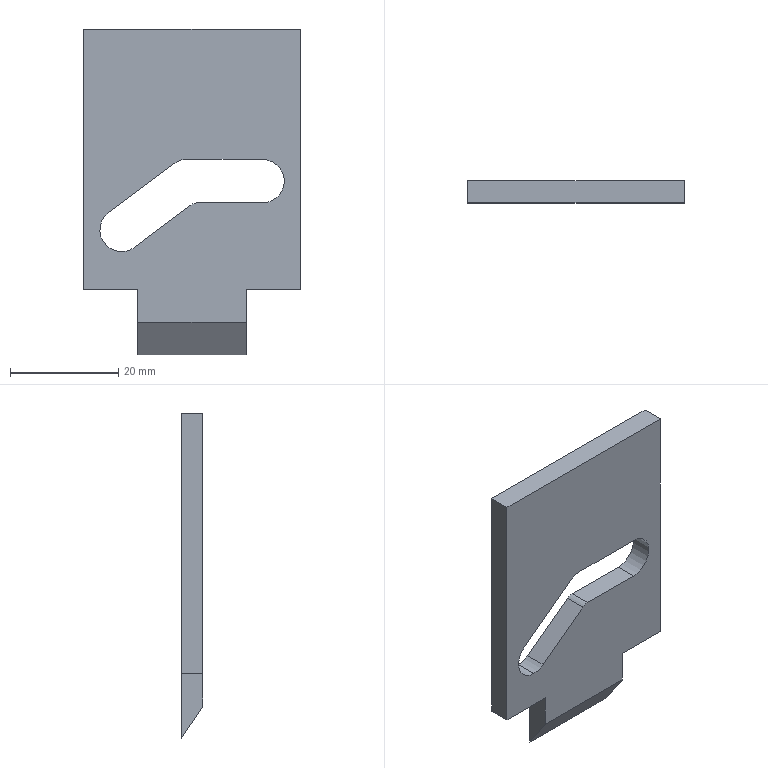Part | SolidWorks | features BaseBody 1 | 1 solid | 19 faces | box 40 x 4 x 60 mm | volume 7271 mm3 | plane 14 | cylinder 5 | commonest cylinder face diameters 8 x4 4 x1
STEP:
#1=CARTESIAN_POINT('',(-13.,4.,-17.));
#2=VERTEX_POINT('',#1);
#3=CARTESIAN_POINT('',(-10.6,4.,-16.2));
#4=VERTEX_POINT('',#3);
#5=CARTESIAN_POINT('',(-13.,4.,-13.));
#6=DIRECTION('',(0.,-1.,0.));
#7=DIRECTION('',(0.,0.,-1.));
#8=AXIS2_PLACEMENT_3D('',#5,#6,#7);
#9=CIRCLE('',#8,4.);
#10=EDGE_CURVE('',#2,#4,#9,.T.);
#11=ORIENTED_EDGE('',*,*,#10,.F.);
#12=CARTESIAN_POINT('',(-13.,0.,-17.));
#13=VERTEX_POINT('',#12);
#14=CARTESIAN_POINT('',(-13.,4.,-17.));
#15=DIRECTION('',(0.,-1.,0.));
#16=VECTOR('',#15,1000.);
#17=LINE('',#14,#16);
#18=EDGE_CURVE('',#2,#13,#17,.T.);
#19=ORIENTED_EDGE('',*,*,#18,.T.);
#20=CARTESIAN_POINT('',(-10.6,0.,-16.2));
#21=VERTEX_POINT('',#20);
#22=CARTESIAN_POINT('',(-13.,0.,-13.));
#23=DIRECTION('',(0.,1.,0.));
#24=DIRECTION('',(0.,0.,-1.));
#25=AXIS2_PLACEMENT_3D('',#22,#23,#24);
#26=CIRCLE('',#25,4.);
#27=EDGE_CURVE('',#21,#13,#26,.T.);
#28=ORIENTED_EDGE('',*,*,#27,.F.);
#29=CARTESIAN_POINT('',(-10.6,4.,-16.2));
#30=DIRECTION('',(0.,-1.,0.));
#31=VECTOR('',#30,1000.);
#32=LINE('',#29,#31);
#33=EDGE_CURVE('',#4,#21,#32,.T.);
#34=ORIENTED_EDGE('',*,*,#33,.F.);
#35=EDGE_LOOP('',(#11,#19,#28,#34));
#36=FACE_OUTER_BOUND('',#35,.T.);
#37=CARTESIAN_POINT('',(-13.,4.,-13.));
#38=DIRECTION('',(0.,-1.,0.));
#39=DIRECTION('',(0.,0.,-1.));
#40=AXIS2_PLACEMENT_3D('',#37,#38,#39);
#41=CYLINDRICAL_SURFACE('',#40,4.);
#42=ADVANCED_FACE('',(#36),#41,.F.);
#43=CARTESIAN_POINT('',(-15.4,4.,-9.8));
#44=VERTEX_POINT('',#43);
#45=CARTESIAN_POINT('',(-13.,4.,-13.));
#46=DIRECTION('',(0.,-1.,0.));
#47=DIRECTION('',(0.,0.,-1.));
#48=AXIS2_PLACEMENT_3D('',#45,#46,#47);
#49=CIRCLE('',#48,4.);
#50=EDGE_CURVE('',#44,#2,#49,.T.);
#51=ORIENTED_EDGE('',*,*,#50,.T.);
#52=ORIENTED_EDGE('',*,*,#10,.T.);
#53=CARTESIAN_POINT('',(-0.2,4.,-8.4));
#54=VERTEX_POINT('',#53);
#55=CARTESIAN_POINT('',(-10.6,4.,-16.2));
#56=DIRECTION('',(0.8,0.,0.6));
#57=VECTOR('',#56,1000.);
#58=LINE('',#55,#57);
#59=EDGE_CURVE('',#4,#54,#58,.T.);
#60=ORIENTED_EDGE('',*,*,#59,.T.);
#61=CARTESIAN_POINT('',(1.,4.,-8.));
#62=VERTEX_POINT('',#61);
#63=CARTESIAN_POINT('',(1.,4.,-10.));
#64=DIRECTION('',(0.,-1.,0.));
#65=DIRECTION('',(0.,0.,-1.));
#66=AXIS2_PLACEMENT_3D('',#63,#64,#65);
#67=CIRCLE('',#66,2.);
#68=EDGE_CURVE('',#62,#54,#67,.T.);
#69=ORIENTED_EDGE('',*,*,#68,.F.);
#70=CARTESIAN_POINT('',(13.,4.,-8.));
#71=VERTEX_POINT('',#70);
#72=CARTESIAN_POINT('',(0.,4.,-8.));
#73=DIRECTION('',(1.,0.,0.));
#74=VECTOR('',#73,1000.);
#75=LINE('',#72,#74);
#76=EDGE_CURVE('',#62,#71,#75,.T.);
#77=ORIENTED_EDGE('',*,*,#76,.T.);
#78=CARTESIAN_POINT('',(13.,4.,0.));
#79=VERTEX_POINT('',#78);
#80=CARTESIAN_POINT('',(13.,4.,-4.));
#81=DIRECTION('',(0.,-1.,0.));
#82=DIRECTION('',(0.,0.,-1.));
#83=AXIS2_PLACEMENT_3D('',#80,#81,#82);
#84=CIRCLE('',#83,4.);
#85=EDGE_CURVE('',#71,#79,#84,.T.);
#86=ORIENTED_EDGE('',*,*,#85,.T.);
#87=CARTESIAN_POINT('',(-1.,4.,0.));
#88=VERTEX_POINT('',#87);
#89=CARTESIAN_POINT('',(0.,4.,0.));
#90=DIRECTION('',(-1.,0.,0.));
#91=VECTOR('',#90,1000.);
#92=LINE('',#89,#91);
#93=EDGE_CURVE('',#79,#88,#92,.T.);
#94=ORIENTED_EDGE('',*,*,#93,.T.);
#95=CARTESIAN_POINT('',(-3.4,4.,-0.8));
#96=VERTEX_POINT('',#95);
#97=CARTESIAN_POINT('',(-1.,4.,-4.));
#98=DIRECTION('',(0.,-1.,0.));
#99=DIRECTION('',(0.,0.,-1.));
#100=AXIS2_PLACEMENT_3D('',#97,#98,#99);
#101=CIRCLE('',#100,4.);
#102=EDGE_CURVE('',#88,#96,#101,.T.);
#103=ORIENTED_EDGE('',*,*,#102,.T.);
#104=CARTESIAN_POINT('',(-3.4,4.,-0.8));
#105=DIRECTION('',(-0.8,0.,-0.6));
#106=VECTOR('',#105,1000.);
#107=LINE('',#104,#106);
#108=EDGE_CURVE('',#96,#44,#107,.T.);
#109=ORIENTED_EDGE('',*,*,#108,.T.);
#110=EDGE_LOOP('',(#51,#52,#60,#69,#77,#86,#94,#103,#109));
#111=FACE_BOUND('',#110,.T.);
#112=CARTESIAN_POINT('',(20.,4.,24.));
#113=VERTEX_POINT('',#112);
#114=CARTESIAN_POINT('',(20.,4.,-24.));
#115=VERTEX_POINT('',#114);
#116=CARTESIAN_POINT('',(20.,4.,0.));
#117=DIRECTION('',(0.,0.,-1.));
#118=VECTOR('',#117,1000.);
#119=LINE('',#116,#118);
#120=EDGE_CURVE('',#113,#115,#119,.T.);
#121=ORIENTED_EDGE('',*,*,#120,.T.);
#122=CARTESIAN_POINT('',(10.,4.,-24.));
#123=VERTEX_POINT('',#122);
#124=CARTESIAN_POINT('',(0.,4.,-24.));
#125=DIRECTION('',(-1.,0.,0.));
#126=VECTOR('',#125,1000.);
#127=LINE('',#124,#126);
#128=EDGE_CURVE('',#115,#123,#127,.T.);
#129=ORIENTED_EDGE('',*,*,#128,.T.);
#130=CARTESIAN_POINT('',(10.,4.,-36.));
#131=VERTEX_POINT('',#130);
#132=CARTESIAN_POINT('',(10.,4.,0.));
#133=DIRECTION('',(0.,0.,-1.));
#134=VECTOR('',#133,1000.);
#135=LINE('',#132,#134);
#136=EDGE_CURVE('',#123,#131,#135,.T.);
#137=ORIENTED_EDGE('',*,*,#136,.T.);
#138=CARTESIAN_POINT('',(-10.,4.,-36.));
#139=VERTEX_POINT('',#138);
#140=CARTESIAN_POINT('',(0.,4.,-36.));
#141=DIRECTION('',(-1.,0.,0.));
#142=VECTOR('',#141,1000.);
#143=LINE('',#140,#142);
#144=EDGE_CURVE('',#131,#139,#143,.T.);
#145=ORIENTED_EDGE('',*,*,#144,.T.);
#146=CARTESIAN_POINT('',(-10.,4.,-24.));
#147=VERTEX_POINT('',#146);
#148=CARTESIAN_POINT('',(-10.,4.,0.));
#149=DIRECTION('',(0.,0.,1.));
#150=VECTOR('',#149,1000.);
#151=LINE('',#148,#150);
#152=EDGE_CURVE('',#139,#147,#151,.T.);
#153=ORIENTED_EDGE('',*,*,#152,.T.);
#154=CARTESIAN_POINT('',(-20.,4.,-24.));
#155=VERTEX_POINT('',#154);
#156=CARTESIAN_POINT('',(0.,4.,-24.));
#157=DIRECTION('',(-1.,0.,0.));
#158=VECTOR('',#157,1000.);
#159=LINE('',#156,#158);
#160=EDGE_CURVE('',#147,#155,#159,.T.);
#161=ORIENTED_EDGE('',*,*,#160,.T.);
#162=CARTESIAN_POINT('',(-20.,4.,24.));
#163=VERTEX_POINT('',#162);
#164=CARTESIAN_POINT('',(-20.,4.,0.));
#165=DIRECTION('',(0.,0.,1.));
#166=VECTOR('',#165,1000.);
#167=LINE('',#164,#166);
#168=EDGE_CURVE('',#155,#163,#167,.T.);
#169=ORIENTED_EDGE('',*,*,#168,.T.);
#170=CARTESIAN_POINT('',(0.,4.,24.));
#171=DIRECTION('',(1.,0.,0.));
#172=VECTOR('',#171,1000.);
#173=LINE('',#170,#172);
#174=EDGE_CURVE('',#163,#113,#173,.T.);
#175=ORIENTED_EDGE('',*,*,#174,.T.);
#176=EDGE_LOOP('',(#121,#129,#137,#145,#153,#161,#169,#175));
#177=FACE_OUTER_BOUND('',#176,.T.);
#178=CARTESIAN_POINT('',(0.,4.,0.));
#179=DIRECTION('',(0.,1.,0.));
#180=DIRECTION('',(0.,0.,1.));
#181=AXIS2_PLACEMENT_3D('',#178,#179,#180);
#182=PLANE('',#181);
#183=ADVANCED_FACE('',(#111,#177),#182,.T.);
#184=ORIENTED_EDGE('',*,*,#18,.F.);
#185=ORIENTED_EDGE('',*,*,#50,.F.);
#186=CARTESIAN_POINT('',(-15.4,0.,-9.8));
#187=VERTEX_POINT('',#186);
#188=CARTESIAN_POINT('',(-15.4,4.,-9.8));
#189=DIRECTION('',(0.,1.,0.));
#190=VECTOR('',#189,1000.);
#191=LINE('',#188,#190);
#192=EDGE_CURVE('',#187,#44,#191,.T.);
#193=ORIENTED_EDGE('',*,*,#192,.F.);
#194=CARTESIAN_POINT('',(-13.,0.,-13.));
#195=DIRECTION('',(0.,1.,0.));
#196=DIRECTION('',(0.,0.,-1.));
#197=AXIS2_PLACEMENT_3D('',#194,#195,#196);
#198=CIRCLE('',#197,4.);
#199=EDGE_CURVE('',#13,#187,#198,.T.);
#200=ORIENTED_EDGE('',*,*,#199,.F.);
#201=EDGE_LOOP('',(#184,#185,#193,#200));
#202=FACE_OUTER_BOUND('',#201,.T.);
#203=CARTESIAN_POINT('',(-13.,4.,-13.));
#204=DIRECTION('',(0.,-1.,0.));
#205=DIRECTION('',(0.,0.,-1.));
#206=AXIS2_PLACEMENT_3D('',#203,#204,#205);
#207=CYLINDRICAL_SURFACE('',#206,4.);
#208=ADVANCED_FACE('',(#202),#207,.F.);
#209=ORIENTED_EDGE('',*,*,#192,.T.);
#210=ORIENTED_EDGE('',*,*,#108,.F.);
#211=CARTESIAN_POINT('',(-3.4,0.,-0.8));
#212=VERTEX_POINT('',#211);
#213=CARTESIAN_POINT('',(-3.4,4.,-0.8));
#214=DIRECTION('',(0.,1.,0.));
#215=VECTOR('',#214,1000.);
#216=LINE('',#213,#215);
#217=EDGE_CURVE('',#212,#96,#216,.T.);
#218=ORIENTED_EDGE('',*,*,#217,.F.);
#219=CARTESIAN_POINT('',(-0.84,0.,1.12));
#220=DIRECTION('',(0.8,0.,0.6));
#221=VECTOR('',#220,1000.);
#222=LINE('',#219,#221);
#223=EDGE_CURVE('',#187,#212,#222,.T.);
#224=ORIENTED_EDGE('',*,*,#223,.F.);
#225=EDGE_LOOP('',(#209,#210,#218,#224));
#226=FACE_OUTER_BOUND('',#225,.T.);
#227=CARTESIAN_POINT('',(-0.84,4.,1.12));
#228=DIRECTION('',(-0.6,0.,0.8));
#229=DIRECTION('',(0.8,0.,0.6));
#230=AXIS2_PLACEMENT_3D('',#227,#228,#229);
#231=PLANE('',#230);
#232=ADVANCED_FACE('',(#226),#231,.F.);
#233=ORIENTED_EDGE('',*,*,#217,.T.);
#234=ORIENTED_EDGE('',*,*,#102,.F.);
#235=CARTESIAN_POINT('',(-1.,0.,0.));
#236=VERTEX_POINT('',#235);
#237=CARTESIAN_POINT('',(-1.,4.,0.));
#238=DIRECTION('',(0.,1.,0.));
#239=VECTOR('',#238,1000.);
#240=LINE('',#237,#239);
#241=EDGE_CURVE('',#236,#88,#240,.T.);
#242=ORIENTED_EDGE('',*,*,#241,.F.);
#243=CARTESIAN_POINT('',(-1.,0.,-4.));
#244=DIRECTION('',(0.,1.,0.));
#245=DIRECTION('',(0.,0.,-1.));
#246=AXIS2_PLACEMENT_3D('',#243,#244,#245);
#247=CIRCLE('',#246,4.);
#248=EDGE_CURVE('',#212,#236,#247,.T.);
#249=ORIENTED_EDGE('',*,*,#248,.F.);
#250=EDGE_LOOP('',(#233,#234,#242,#249));
#251=FACE_OUTER_BOUND('',#250,.T.);
#252=CARTESIAN_POINT('',(-1.,4.,-4.));
#253=DIRECTION('',(0.,-1.,0.));
#254=DIRECTION('',(0.,0.,-1.));
#255=AXIS2_PLACEMENT_3D('',#252,#253,#254);
#256=CYLINDRICAL_SURFACE('',#255,4.);
#257=ADVANCED_FACE('',(#251),#256,.F.);
#258=ORIENTED_EDGE('',*,*,#93,.F.);
#259=CARTESIAN_POINT('',(13.,0.,0.));
#260=VERTEX_POINT('',#259);
#261=CARTESIAN_POINT('',(13.,4.,0.));
#262=DIRECTION('',(0.,-1.,0.));
#263=VECTOR('',#262,1000.);
#264=LINE('',#261,#263);
#265=EDGE_CURVE('',#79,#260,#264,.T.);
#266=ORIENTED_EDGE('',*,*,#265,.T.);
#267=CARTESIAN_POINT('',(0.,0.,0.));
#268=DIRECTION('',(-1.,0.,0.));
#269=VECTOR('',#268,1000.);
#270=LINE('',#267,#269);
#271=EDGE_CURVE('',#260,#236,#270,.T.);
#272=ORIENTED_EDGE('',*,*,#271,.T.);
#273=ORIENTED_EDGE('',*,*,#241,.T.);
#274=EDGE_LOOP('',(#258,#266,#272,#273));
#275=FACE_OUTER_BOUND('',#274,.T.);
#276=CARTESIAN_POINT('',(0.,4.,0.));
#277=DIRECTION('',(0.,0.,-1.));
#278=DIRECTION('',(-1.,0.,0.));
#279=AXIS2_PLACEMENT_3D('',#276,#277,#278);
#280=PLANE('',#279);
#281=ADVANCED_FACE('',(#275),#280,.T.);
#282=ORIENTED_EDGE('',*,*,#265,.F.);
#283=ORIENTED_EDGE('',*,*,#85,.F.);
#284=CARTESIAN_POINT('',(13.,0.,-8.));
#285=VERTEX_POINT('',#284);
#286=CARTESIAN_POINT('',(13.,4.,-8.));
#287=DIRECTION('',(0.,1.,0.));
#288=VECTOR('',#287,1000.);
#289=LINE('',#286,#288);
#290=EDGE_CURVE('',#285,#71,#289,.T.);
#291=ORIENTED_EDGE('',*,*,#290,.F.);
#292=CARTESIAN_POINT('',(13.,0.,-4.));
#293=DIRECTION('',(0.,1.,0.));
#294=DIRECTION('',(0.,0.,-1.));
#295=AXIS2_PLACEMENT_3D('',#292,#293,#294);
#296=CIRCLE('',#295,4.);
#297=EDGE_CURVE('',#260,#285,#296,.T.);
#298=ORIENTED_EDGE('',*,*,#297,.F.);
#299=EDGE_LOOP('',(#282,#283,#291,#298));
#300=FACE_OUTER_BOUND('',#299,.T.);
#301=CARTESIAN_POINT('',(13.,4.,-4.));
#302=DIRECTION('',(0.,-1.,0.));
#303=DIRECTION('',(0.,0.,-1.));
#304=AXIS2_PLACEMENT_3D('',#301,#302,#303);
#305=CYLINDRICAL_SURFACE('',#304,4.);
#306=ADVANCED_FACE('',(#300),#305,.F.);
#307=ORIENTED_EDGE('',*,*,#290,.T.);
#308=ORIENTED_EDGE('',*,*,#76,.F.);
#309=CARTESIAN_POINT('',(1.,0.,-8.));
#310=VERTEX_POINT('',#309);
#311=CARTESIAN_POINT('',(1.,4.,-8.));
#312=DIRECTION('',(0.,1.,0.));
#313=VECTOR('',#312,1000.);
#314=LINE('',#311,#313);
#315=EDGE_CURVE('',#310,#62,#314,.T.);
#316=ORIENTED_EDGE('',*,*,#315,.F.);
#317=CARTESIAN_POINT('',(0.,0.,-8.));
#318=DIRECTION('',(-1.,0.,0.));
#319=VECTOR('',#318,1000.);
#320=LINE('',#317,#319);
#321=EDGE_CURVE('',#285,#310,#320,.T.);
#322=ORIENTED_EDGE('',*,*,#321,.F.);
#323=EDGE_LOOP('',(#307,#308,#316,#322));
#324=FACE_OUTER_BOUND('',#323,.T.);
#325=CARTESIAN_POINT('',(0.,4.,-8.));
#326=DIRECTION('',(0.,0.,-1.));
#327=DIRECTION('',(-1.,0.,0.));
#328=AXIS2_PLACEMENT_3D('',#325,#326,#327);
#329=PLANE('',#328);
#330=ADVANCED_FACE('',(#324),#329,.F.);
#331=ORIENTED_EDGE('',*,*,#59,.F.);
#332=ORIENTED_EDGE('',*,*,#33,.T.);
#333=CARTESIAN_POINT('',(-0.2,0.,-8.4));
#334=VERTEX_POINT('',#333);
#335=CARTESIAN_POINT('',(3.96,0.,-5.28));
#336=DIRECTION('',(0.8,0.,0.6));
#337=VECTOR('',#336,1000.);
#338=LINE('',#335,#337);
#339=EDGE_CURVE('',#21,#334,#338,.T.);
#340=ORIENTED_EDGE('',*,*,#339,.T.);
#341=CARTESIAN_POINT('',(-0.2,4.,-8.4));
#342=DIRECTION('',(0.,1.,0.));
#343=VECTOR('',#342,1000.);
#344=LINE('',#341,#343);
#345=EDGE_CURVE('',#334,#54,#344,.T.);
#346=ORIENTED_EDGE('',*,*,#345,.T.);
#347=EDGE_LOOP('',(#331,#332,#340,#346));
#348=FACE_OUTER_BOUND('',#347,.T.);
#349=CARTESIAN_POINT('',(3.96,4.,-5.28));
#350=DIRECTION('',(-0.6,0.,0.8));
#351=DIRECTION('',(0.8,0.,0.6));
#352=AXIS2_PLACEMENT_3D('',#349,#350,#351);
#353=PLANE('',#352);
#354=ADVANCED_FACE('',(#348),#353,.T.);
#355=ORIENTED_EDGE('',*,*,#128,.F.);
#356=CARTESIAN_POINT('',(20.,0.,-24.));
#357=VERTEX_POINT('',#356);
#358=CARTESIAN_POINT('',(20.,4.,-24.));
#359=DIRECTION('',(0.,-1.,0.));
#360=VECTOR('',#359,1000.);
#361=LINE('',#358,#360);
#362=EDGE_CURVE('',#115,#357,#361,.T.);
#363=ORIENTED_EDGE('',*,*,#362,.T.);
#364=CARTESIAN_POINT('',(10.,0.,-24.));
#365=VERTEX_POINT('',#364);
#366=CARTESIAN_POINT('',(0.,0.,-24.));
#367=DIRECTION('',(-1.,0.,0.));
#368=VECTOR('',#367,1000.);
#369=LINE('',#366,#368);
#370=EDGE_CURVE('',#357,#365,#369,.T.);
#371=ORIENTED_EDGE('',*,*,#370,.T.);
#372=CARTESIAN_POINT('',(10.,4.,-24.));
#373=DIRECTION('',(0.,1.,0.));
#374=VECTOR('',#373,1000.);
#375=LINE('',#372,#374);
#376=EDGE_CURVE('',#365,#123,#375,.T.);
#377=ORIENTED_EDGE('',*,*,#376,.T.);
#378=EDGE_LOOP('',(#355,#363,#371,#377));
#379=FACE_OUTER_BOUND('',#378,.T.);
#380=CARTESIAN_POINT('',(0.,4.,-24.));
#381=DIRECTION('',(0.,0.,-1.));
#382=DIRECTION('',(-1.,0.,0.));
#383=AXIS2_PLACEMENT_3D('',#380,#381,#382);
#384=PLANE('',#383);
#385=ADVANCED_FACE('',(#379),#384,.T.);
#386=ORIENTED_EDGE('',*,*,#362,.F.);
#387=ORIENTED_EDGE('',*,*,#120,.F.);
#388=CARTESIAN_POINT('',(20.,0.,24.));
#389=VERTEX_POINT('',#388);
#390=CARTESIAN_POINT('',(20.,4.,24.));
#391=DIRECTION('',(0.,1.,0.));
#392=VECTOR('',#391,1000.);
#393=LINE('',#390,#392);
#394=EDGE_CURVE('',#389,#113,#393,.T.);
#395=ORIENTED_EDGE('',*,*,#394,.F.);
#396=CARTESIAN_POINT('',(20.,0.,0.));
#397=DIRECTION('',(0.,0.,1.));
#398=VECTOR('',#397,1000.);
#399=LINE('',#396,#398);
#400=EDGE_CURVE('',#357,#389,#399,.T.);
#401=ORIENTED_EDGE('',*,*,#400,.F.);
#402=EDGE_LOOP('',(#386,#387,#395,#401));
#403=FACE_OUTER_BOUND('',#402,.T.);
#404=CARTESIAN_POINT('',(20.,4.,0.));
#405=DIRECTION('',(-1.,0.,0.));
#406=DIRECTION('',(0.,0.,1.));
#407=AXIS2_PLACEMENT_3D('',#404,#405,#406);
#408=PLANE('',#407);
#409=ADVANCED_FACE('',(#403),#408,.F.);
#410=ORIENTED_EDGE('',*,*,#394,.T.);
#411=ORIENTED_EDGE('',*,*,#174,.F.);
#412=CARTESIAN_POINT('',(-20.,0.,24.));
#413=VERTEX_POINT('',#412);
#414=CARTESIAN_POINT('',(-20.,4.,24.));
#415=DIRECTION('',(0.,1.,0.));
#416=VECTOR('',#415,1000.);
#417=LINE('',#414,#416);
#418=EDGE_CURVE('',#413,#163,#417,.T.);
#419=ORIENTED_EDGE('',*,*,#418,.F.);
#420=CARTESIAN_POINT('',(0.,0.,24.));
#421=DIRECTION('',(-1.,0.,0.));
#422=VECTOR('',#421,1000.);
#423=LINE('',#420,#422);
#424=EDGE_CURVE('',#389,#413,#423,.T.);
#425=ORIENTED_EDGE('',*,*,#424,.F.);
#426=EDGE_LOOP('',(#410,#411,#419,#425));
#427=FACE_OUTER_BOUND('',#426,.T.);
#428=CARTESIAN_POINT('',(0.,4.,24.));
#429=DIRECTION('',(0.,0.,-1.));
#430=DIRECTION('',(-1.,0.,0.));
#431=AXIS2_PLACEMENT_3D('',#428,#429,#430);
#432=PLANE('',#431);
#433=ADVANCED_FACE('',(#427),#432,.F.);
#434=ORIENTED_EDGE('',*,*,#168,.F.);
#435=CARTESIAN_POINT('',(-20.,0.,-24.));
#436=VERTEX_POINT('',#435);
#437=CARTESIAN_POINT('',(-20.,4.,-24.));
#438=DIRECTION('',(0.,-1.,0.));
#439=VECTOR('',#438,1000.);
#440=LINE('',#437,#439);
#441=EDGE_CURVE('',#155,#436,#440,.T.);
#442=ORIENTED_EDGE('',*,*,#441,.T.);
#443=CARTESIAN_POINT('',(-20.,0.,0.));
#444=DIRECTION('',(0.,0.,1.));
#445=VECTOR('',#444,1000.);
#446=LINE('',#443,#445);
#447=EDGE_CURVE('',#436,#413,#446,.T.);
#448=ORIENTED_EDGE('',*,*,#447,.T.);
#449=ORIENTED_EDGE('',*,*,#418,.T.);
#450=EDGE_LOOP('',(#434,#442,#448,#449));
#451=FACE_OUTER_BOUND('',#450,.T.);
#452=CARTESIAN_POINT('',(-20.,4.,0.));
#453=DIRECTION('',(-1.,0.,0.));
#454=DIRECTION('',(0.,0.,1.));
#455=AXIS2_PLACEMENT_3D('',#452,#453,#454);
#456=PLANE('',#455);
#457=ADVANCED_FACE('',(#451),#456,.T.);
#458=ORIENTED_EDGE('',*,*,#160,.F.);
#459=CARTESIAN_POINT('',(-10.,0.,-24.));
#460=VERTEX_POINT('',#459);
#461=CARTESIAN_POINT('',(-10.,4.,-24.));
#462=DIRECTION('',(0.,-1.,0.));
#463=VECTOR('',#462,1000.);
#464=LINE('',#461,#463);
#465=EDGE_CURVE('',#147,#460,#464,.T.);
#466=ORIENTED_EDGE('',*,*,#465,.T.);
#467=CARTESIAN_POINT('',(0.,0.,-24.));
#468=DIRECTION('',(-1.,0.,0.));
#469=VECTOR('',#468,1000.);
#470=LINE('',#467,#469);
#471=EDGE_CURVE('',#460,#436,#470,.T.);
#472=ORIENTED_EDGE('',*,*,#471,.T.);
#473=ORIENTED_EDGE('',*,*,#441,.F.);
#474=EDGE_LOOP('',(#458,#466,#472,#473));
#475=FACE_OUTER_BOUND('',#474,.T.);
#476=CARTESIAN_POINT('',(0.,4.,-24.));
#477=DIRECTION('',(0.,0.,-1.));
#478=DIRECTION('',(-1.,0.,0.));
#479=AXIS2_PLACEMENT_3D('',#476,#477,#478);
#480=PLANE('',#479);
#481=ADVANCED_FACE('',(#475),#480,.T.);
#482=CARTESIAN_POINT('',(-10.,0.,-30.));
#483=VERTEX_POINT('',#482);
#484=CARTESIAN_POINT('',(-10.,0.,-30.));
#485=DIRECTION('',(0.,0.5547,-0.8321));
#486=VECTOR('',#485,1000.);
#487=LINE('',#484,#486);
#488=EDGE_CURVE('',#483,#139,#487,.T.);
#489=ORIENTED_EDGE('',*,*,#488,.F.);
#490=CARTESIAN_POINT('',(-10.,0.,0.));
#491=DIRECTION('',(0.,0.,-1.));
#492=VECTOR('',#491,1000.);
#493=LINE('',#490,#492);
#494=EDGE_CURVE('',#460,#483,#493,.T.);
#495=ORIENTED_EDGE('',*,*,#494,.F.);
#496=ORIENTED_EDGE('',*,*,#465,.F.);
#497=ORIENTED_EDGE('',*,*,#152,.F.);
#498=EDGE_LOOP('',(#489,#495,#496,#497));
#499=FACE_OUTER_BOUND('',#498,.T.);
#500=CARTESIAN_POINT('',(-10.,4.,0.));
#501=DIRECTION('',(1.,0.,0.));
#502=DIRECTION('',(0.,0.,-1.));
#503=AXIS2_PLACEMENT_3D('',#500,#501,#502);
#504=PLANE('',#503);
#505=ADVANCED_FACE('',(#499),#504,.F.);
#506=CARTESIAN_POINT('',(10.,0.,-30.));
#507=VERTEX_POINT('',#506);
#508=CARTESIAN_POINT('',(20.,0.,-30.));
#509=DIRECTION('',(1.,0.,0.));
#510=VECTOR('',#509,1000.);
#511=LINE('',#508,#510);
#512=EDGE_CURVE('',#483,#507,#511,.T.);
#513=ORIENTED_EDGE('',*,*,#512,.F.);
#514=ORIENTED_EDGE('',*,*,#488,.T.);
#515=ORIENTED_EDGE('',*,*,#144,.F.);
#516=CARTESIAN_POINT('',(10.,4.,-36.));
#517=DIRECTION('',(0.,0.5547,-0.8321));
#518=VECTOR('',#517,1000.);
#519=LINE('',#516,#518);
#520=EDGE_CURVE('',#507,#131,#519,.T.);
#521=ORIENTED_EDGE('',*,*,#520,.F.);
#522=EDGE_LOOP('',(#513,#514,#515,#521));
#523=FACE_OUTER_BOUND('',#522,.T.);
#524=CARTESIAN_POINT('',(20.,4.,-36.));
#525=DIRECTION('',(0.,0.8321,0.5547));
#526=DIRECTION('',(0.,-0.5547,0.8321));
#527=AXIS2_PLACEMENT_3D('',#524,#525,#526);
#528=PLANE('',#527);
#529=ADVANCED_FACE('',(#523),#528,.F.);
#530=ORIENTED_EDGE('',*,*,#376,.F.);
#531=CARTESIAN_POINT('',(10.,0.,0.));
#532=DIRECTION('',(0.,0.,-1.));
#533=VECTOR('',#532,1000.);
#534=LINE('',#531,#533);
#535=EDGE_CURVE('',#365,#507,#534,.T.);
#536=ORIENTED_EDGE('',*,*,#535,.T.);
#537=ORIENTED_EDGE('',*,*,#520,.T.);
#538=ORIENTED_EDGE('',*,*,#136,.F.);
#539=EDGE_LOOP('',(#530,#536,#537,#538));
#540=FACE_OUTER_BOUND('',#539,.T.);
#541=CARTESIAN_POINT('',(10.,4.,0.));
#542=DIRECTION('',(1.,0.,0.));
#543=DIRECTION('',(0.,0.,-1.));
#544=AXIS2_PLACEMENT_3D('',#541,#542,#543);
#545=PLANE('',#544);
#546=ADVANCED_FACE('',(#540),#545,.T.);
#547=ORIENTED_EDGE('',*,*,#27,.T.);
#548=ORIENTED_EDGE('',*,*,#199,.T.);
#549=ORIENTED_EDGE('',*,*,#223,.T.);
#550=ORIENTED_EDGE('',*,*,#248,.T.);
#551=ORIENTED_EDGE('',*,*,#271,.F.);
#552=ORIENTED_EDGE('',*,*,#297,.T.);
#553=ORIENTED_EDGE('',*,*,#321,.T.);
#554=CARTESIAN_POINT('',(1.,0.,-10.));
#555=DIRECTION('',(0.,1.,0.));
#556=DIRECTION('',(0.,0.,-1.));
#557=AXIS2_PLACEMENT_3D('',#554,#555,#556);
#558=CIRCLE('',#557,2.);
#559=EDGE_CURVE('',#334,#310,#558,.T.);
#560=ORIENTED_EDGE('',*,*,#559,.F.);
#561=ORIENTED_EDGE('',*,*,#339,.F.);
#562=EDGE_LOOP('',(#547,#548,#549,#550,#551,#552,#553,#560,#561));
#563=FACE_BOUND('',#562,.T.);
#564=ORIENTED_EDGE('',*,*,#512,.T.);
#565=ORIENTED_EDGE('',*,*,#535,.F.);
#566=ORIENTED_EDGE('',*,*,#370,.F.);
#567=ORIENTED_EDGE('',*,*,#400,.T.);
#568=ORIENTED_EDGE('',*,*,#424,.T.);
#569=ORIENTED_EDGE('',*,*,#447,.F.);
#570=ORIENTED_EDGE('',*,*,#471,.F.);
#571=ORIENTED_EDGE('',*,*,#494,.T.);
#572=EDGE_LOOP('',(#564,#565,#566,#567,#568,#569,#570,#571));
#573=FACE_OUTER_BOUND('',#572,.T.);
#574=CARTESIAN_POINT('',(0.,0.,0.));
#575=DIRECTION('',(0.,1.,0.));
#576=DIRECTION('',(0.,0.,1.));
#577=AXIS2_PLACEMENT_3D('',#574,#575,#576);
#578=PLANE('',#577);
#579=ADVANCED_FACE('',(#563,#573),#578,.F.);
#580=ORIENTED_EDGE('',*,*,#68,.T.);
#581=ORIENTED_EDGE('',*,*,#345,.F.);
#582=ORIENTED_EDGE('',*,*,#559,.T.);
#583=ORIENTED_EDGE('',*,*,#315,.T.);
#584=EDGE_LOOP('',(#580,#581,#582,#583));
#585=FACE_OUTER_BOUND('',#584,.T.);
#586=CARTESIAN_POINT('',(1.,4.,-10.));
#587=DIRECTION('',(0.,-1.,0.));
#588=DIRECTION('',(0.,0.,-1.));
#589=AXIS2_PLACEMENT_3D('',#586,#587,#588);
#590=CYLINDRICAL_SURFACE('',#589,2.);
#591=ADVANCED_FACE('',(#585),#590,.T.);
#592=CLOSED_SHELL('',(#42,#183,#208,#232,#257,#281,#306,#330,#354,#385,#409,#433,#457,#481,#505,#529,#546,#579,#591));
#593=MANIFOLD_SOLID_BREP('',#592);
#594=CARTESIAN_POINT('',(0.,0.,0.));
#595=DIRECTION('',(0.,0.,1.));
#596=DIRECTION('',(1.,0.,0.));
#597=AXIS2_PLACEMENT_3D('',#594,#595,#596);
#598=(LENGTH_UNIT()NAMED_UNIT(*)SI_UNIT(.MILLI.,.METRE.));
#599=UNCERTAINTY_MEASURE_WITH_UNIT(LENGTH_MEASURE(0.00001),#598,'','');
#600=(NAMED_UNIT(*)PLANE_ANGLE_UNIT()SI_UNIT($,.RADIAN.));
#601=(NAMED_UNIT(*)SI_UNIT($,.STERADIAN.)SOLID_ANGLE_UNIT());
#602=(GEOMETRIC_REPRESENTATION_CONTEXT(3)GLOBAL_UNCERTAINTY_ASSIGNED_CONTEXT((#599))GLOBAL_UNIT_ASSIGNED_CONTEXT((#598,#600,#601))REPRESENTATION_CONTEXT('',''));
#603=ADVANCED_BREP_SHAPE_REPRESENTATION('',(#593,#597),#602);